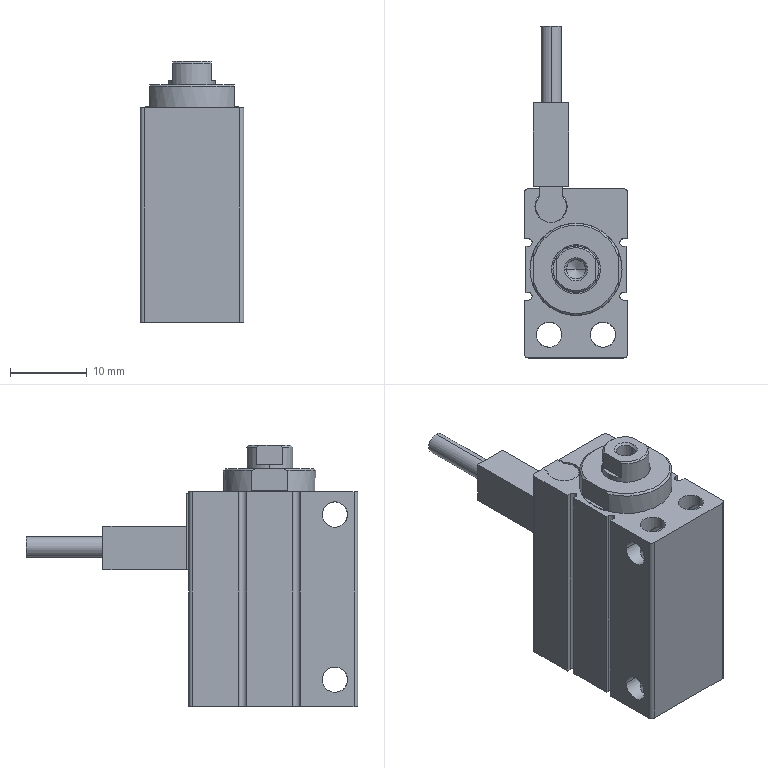Part | SolidWorks | features BaseBody 2 | 2 solids | 114 faces | box 13.5 x 43.2 x 34 mm | volume 7865 mm3 | cylinder 53 | plane 43 | cone 12 | spline 6 | commonest cylinder face diameters 3.3 x24 1 x10 2.46 x6 4.2 x3 2.7 x2 4 x2